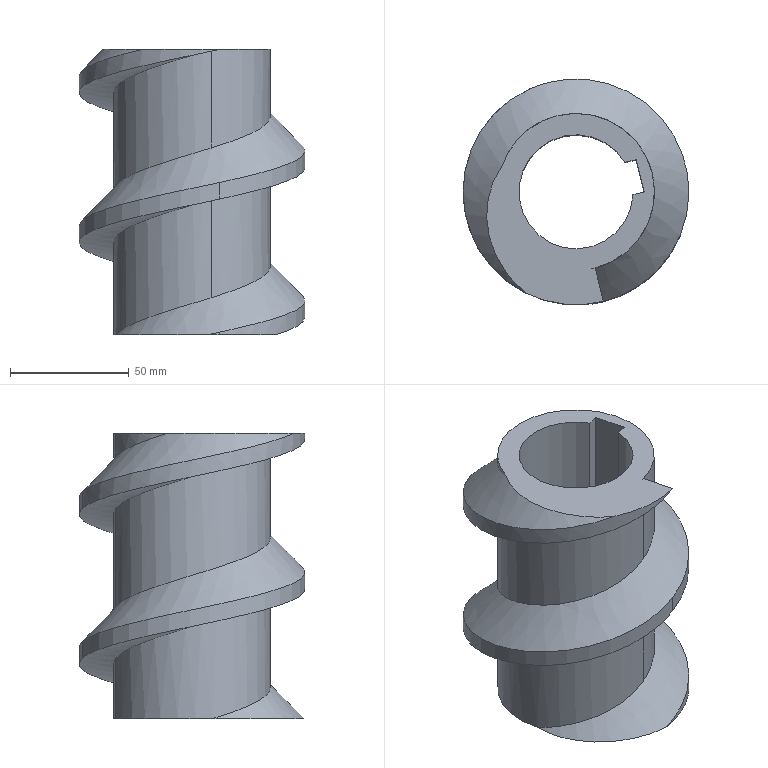Part | SolidWorks | features BaseBody 1, ICE 1, RevCut 1 | 1 solid | 19 faces | box 95 x 95 x 120 mm | volume 282927 mm3 | cylinder 12 | plane 5 | spline 2 | commonest cylinder face diameters 66 x6 95 x5 48 x1